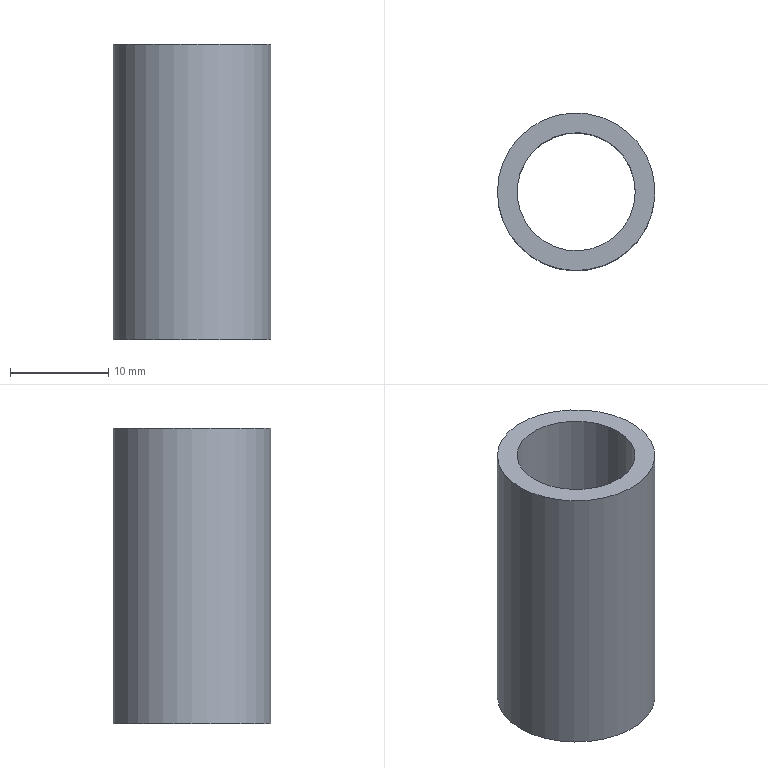Part | NX | features solid 2 | 1 solid | 4 faces | box 16 x 16 x 30 mm | volume 2639 mm3 | plane 2 | cylinder 2 | commonest cylinder face diameters 12 x1 16 x1
STEP:
#1=CARTESIAN_POINT('',(246.,-295.,-90.));
#2=VERTEX_POINT('',#1);
#3=CARTESIAN_POINT('',(240.,-295.,-90.));
#4=DIRECTION('',(0.,0.,1.));
#5=DIRECTION('',(1.,0.,0.));
#6=AXIS2_PLACEMENT_3D('',#3,#4,#5);
#7=CIRCLE('',#6,6.);
#8=EDGE_CURVE('',#2,#2,#7,.T.);
#9=ORIENTED_EDGE('',*,*,#8,.F.);
#10=EDGE_LOOP('',(#9));
#11=FACE_BOUND('',#10,.T.);
#12=CARTESIAN_POINT('',(232.,-295.,-90.));
#13=VERTEX_POINT('',#12);
#14=CARTESIAN_POINT('',(240.,-295.,-90.));
#15=DIRECTION('',(0.,0.,1.));
#16=DIRECTION('',(-1.,0.,0.));
#17=AXIS2_PLACEMENT_3D('',#14,#15,#16);
#18=CIRCLE('',#17,8.);
#19=EDGE_CURVE('',#13,#13,#18,.T.);
#20=ORIENTED_EDGE('',*,*,#19,.T.);
#21=EDGE_LOOP('',(#20));
#22=FACE_BOUND('',#21,.T.);
#23=CARTESIAN_POINT('',(240.,-295.,-90.));
#24=DIRECTION('',(0.,0.,-1.));
#25=DIRECTION('',(-1.,0.,0.));
#26=AXIS2_PLACEMENT_3D('',#23,#24,#25);
#27=PLANE('',#26);
#28=ADVANCED_FACE('',(#11,#22),#27,.F.);
#29=CARTESIAN_POINT('',(246.,-295.,-120.));
#30=VERTEX_POINT('',#29);
#31=CARTESIAN_POINT('',(240.,-295.,-120.));
#32=DIRECTION('',(0.,0.,1.));
#33=DIRECTION('',(1.,0.,0.));
#34=AXIS2_PLACEMENT_3D('',#31,#32,#33);
#35=CIRCLE('',#34,6.);
#36=EDGE_CURVE('',#30,#30,#35,.T.);
#37=ORIENTED_EDGE('',*,*,#36,.T.);
#38=EDGE_LOOP('',(#37));
#39=FACE_BOUND('',#38,.T.);
#40=CARTESIAN_POINT('',(232.,-295.,-120.));
#41=VERTEX_POINT('',#40);
#42=CARTESIAN_POINT('',(240.,-295.,-120.));
#43=DIRECTION('',(0.,0.,1.));
#44=DIRECTION('',(-1.,0.,0.));
#45=AXIS2_PLACEMENT_3D('',#42,#43,#44);
#46=CIRCLE('',#45,8.);
#47=EDGE_CURVE('',#41,#41,#46,.T.);
#48=ORIENTED_EDGE('',*,*,#47,.F.);
#49=EDGE_LOOP('',(#48));
#50=FACE_BOUND('',#49,.T.);
#51=CARTESIAN_POINT('',(240.,-295.,-120.));
#52=DIRECTION('',(0.,0.,-1.));
#53=DIRECTION('',(-1.,0.,0.));
#54=AXIS2_PLACEMENT_3D('',#51,#52,#53);
#55=PLANE('',#54);
#56=ADVANCED_FACE('',(#39,#50),#55,.T.);
#57=ORIENTED_EDGE('',*,*,#8,.T.);
#58=EDGE_LOOP('',(#57));
#59=FACE_BOUND('',#58,.T.);
#60=ORIENTED_EDGE('',*,*,#36,.F.);
#61=EDGE_LOOP('',(#60));
#62=FACE_BOUND('',#61,.T.);
#63=CARTESIAN_POINT('',(240.,-295.,-120.));
#64=DIRECTION('',(0.,0.,1.));
#65=DIRECTION('',(1.,0.,0.));
#66=AXIS2_PLACEMENT_3D('',#63,#64,#65);
#67=CYLINDRICAL_SURFACE('',#66,6.);
#68=ADVANCED_FACE('',(#59,#62),#67,.F.);
#69=ORIENTED_EDGE('',*,*,#19,.F.);
#70=EDGE_LOOP('',(#69));
#71=FACE_BOUND('',#70,.T.);
#72=ORIENTED_EDGE('',*,*,#47,.T.);
#73=EDGE_LOOP('',(#72));
#74=FACE_BOUND('',#73,.T.);
#75=CARTESIAN_POINT('',(240.,-295.,-120.));
#76=DIRECTION('',(0.,0.,1.));
#77=DIRECTION('',(1.,0.,0.));
#78=AXIS2_PLACEMENT_3D('',#75,#76,#77);
#79=CYLINDRICAL_SURFACE('',#78,8.);
#80=ADVANCED_FACE('',(#71,#74),#79,.T.);
#81=CLOSED_SHELL('',(#28,#56,#68,#80));
#82=MANIFOLD_SOLID_BREP('',#81);
#83=(LENGTH_UNIT()NAMED_UNIT(*)SI_UNIT(.MILLI.,.METRE.));
#84=UNCERTAINTY_MEASURE_WITH_UNIT(LENGTH_MEASURE(0.00001),#83,'','');
#85=(NAMED_UNIT(*)PLANE_ANGLE_UNIT()SI_UNIT($,.RADIAN.));
#86=(NAMED_UNIT(*)SI_UNIT($,.STERADIAN.)SOLID_ANGLE_UNIT());
#87=(GEOMETRIC_REPRESENTATION_CONTEXT(3)GLOBAL_UNCERTAINTY_ASSIGNED_CONTEXT((#84))GLOBAL_UNIT_ASSIGNED_CONTEXT((#83,#85,#86))REPRESENTATION_CONTEXT('',''));
#88=ADVANCED_BREP_SHAPE_REPRESENTATION('',(#82),#87);